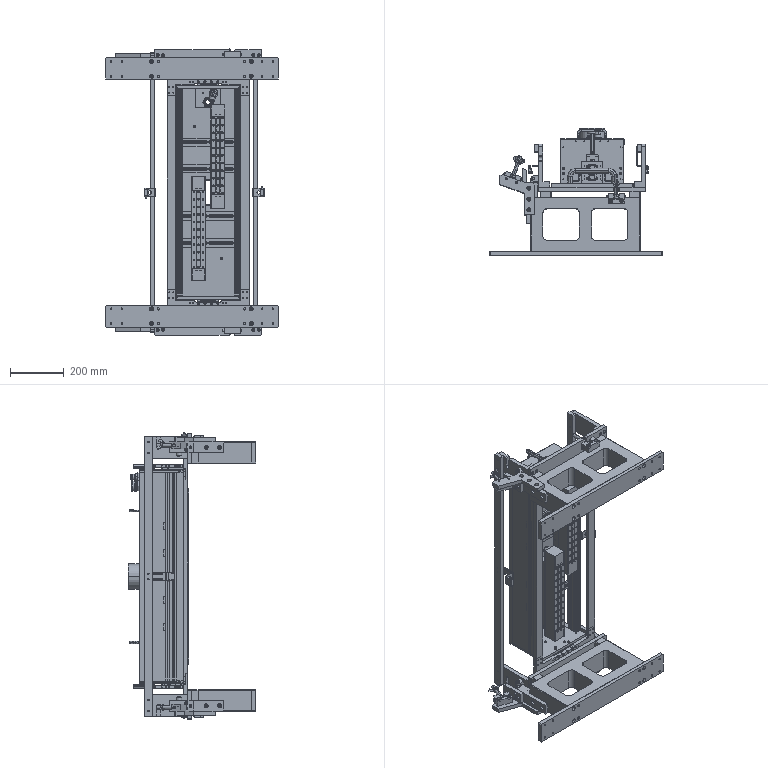Part | SolidWorks | 73 solids | 6581 faces | volume 19986047 mm3 | cylinder 3125 | plane 2179 | cone 1152 | spline 51 | torus 44 | sphere 30 | commonest cylinder face diameters 1 x466 8 x212 3.3 x210 5 x170 10 x146 4.5 x142